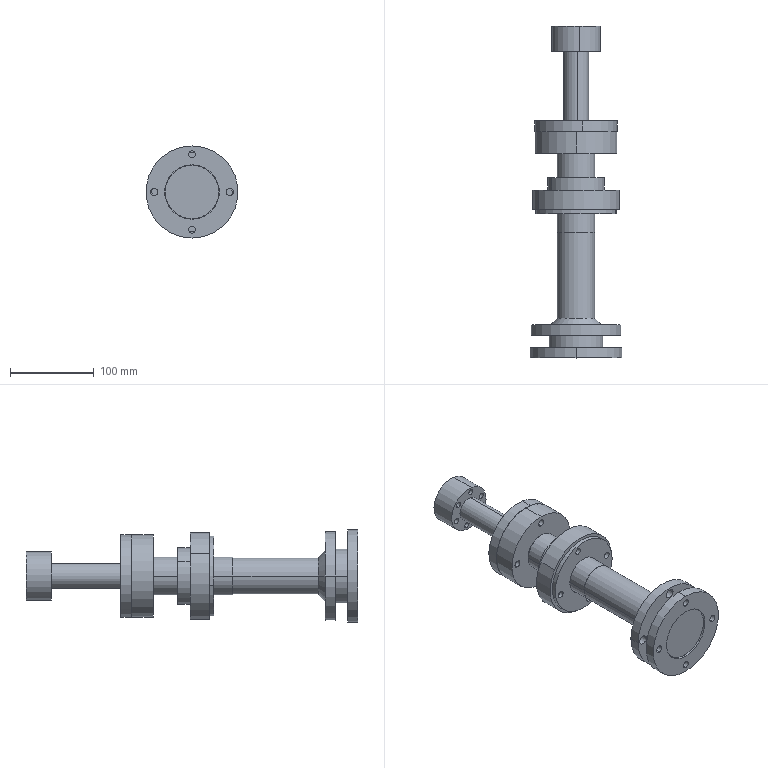Part | SolidWorks | 7 solids | 390 faces | box 110 x 396.3 x 110 mm | volume 1150235 mm3 | spline 166 | cylinder 164 | plane 32 | cone 28 | commonest cylinder face diameters 11 x28 8.5 x24 5 x16 7 x12 6.6 x8 8 x8